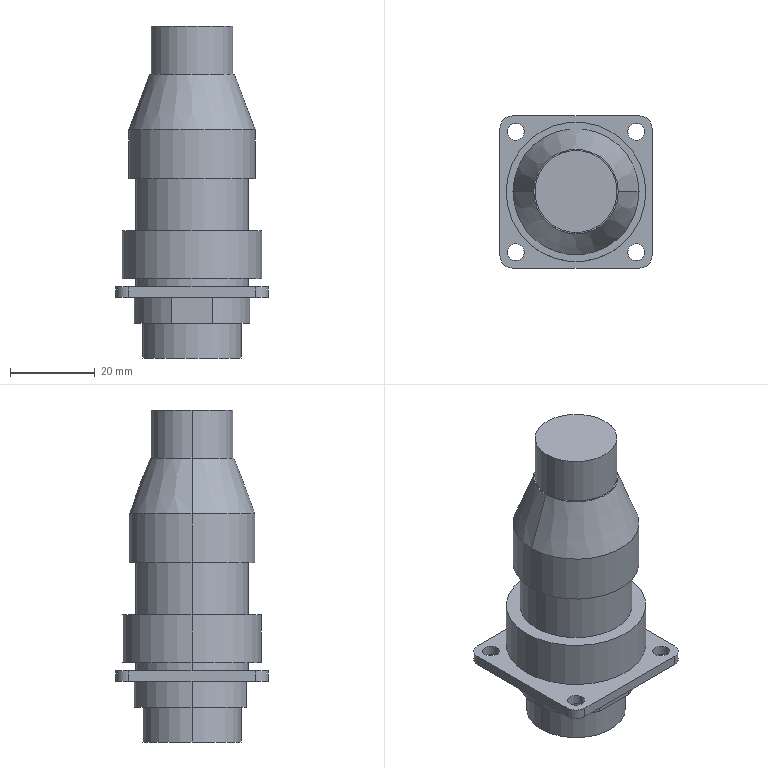Part | STEP file | SMEMA connector | 1 solid | 43 faces | box 36 x 36 x 78.52 mm | volume 45655 mm3 | cylinder 27 | plane 14 | cone 2 | commonest cylinder face diameters 4 x8 6 x4 27.4 x3 19.39 x2 23.38 x2 26.57 x2